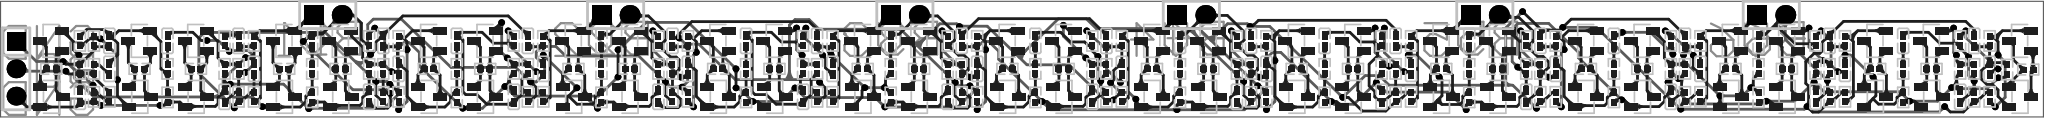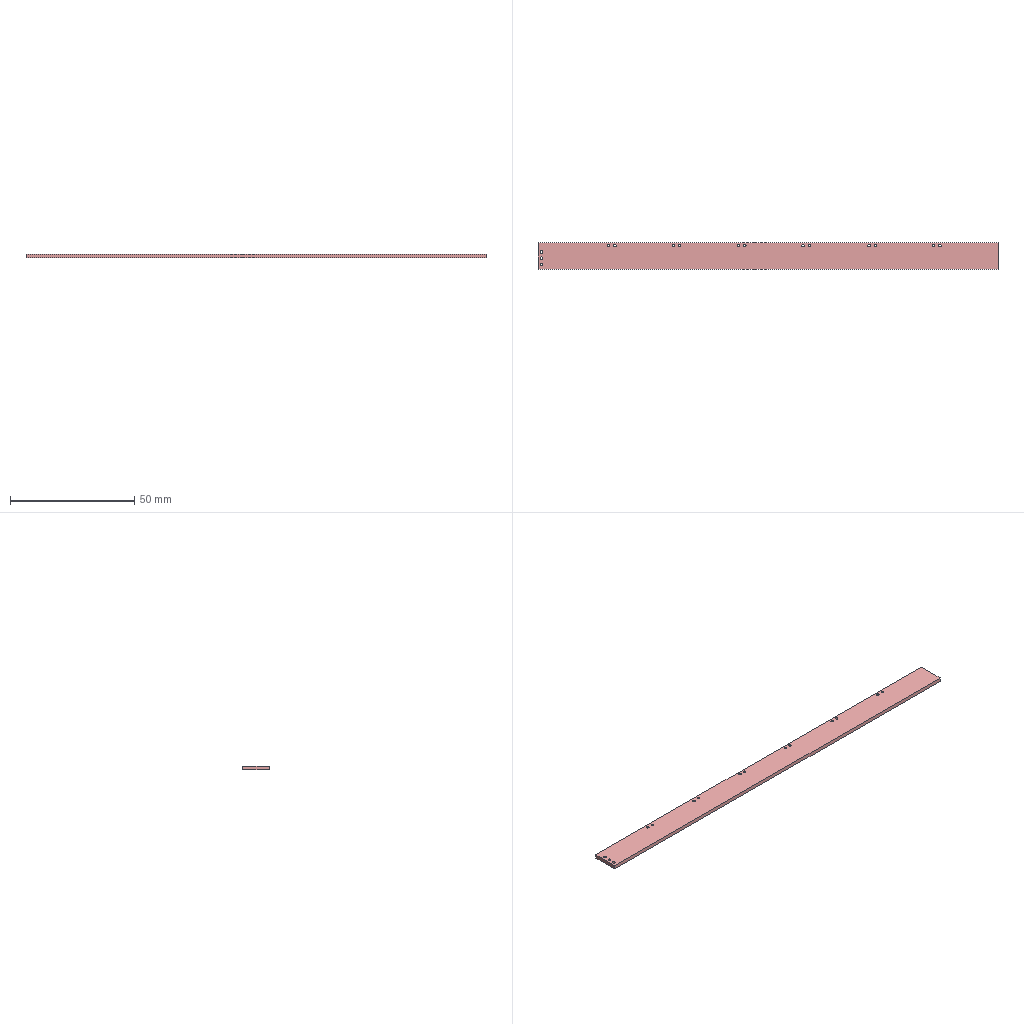Circuit board layout | Altium Designer | box 184.8 x 10.8 x 1.6 mm
Layer stack:
# Altium Designer layer stack of  (unit mm; dielectric type: 0 none, 1 core, 2 prepreg, 3 surface material)
index,name,kind,layer,copper_thickness_mm,dielectric_type,dielectric_thickness_mm,dielectric_material,dielectric_constant
0,Top Paste Mask Layer,other,,,,,,
1,Top Silkscreen Layer,other,,,,,,
2,Top Solder Mask Layer,dielectric,,,3,0.01,,3.3
3,Top Layer,copper,Top Layer,0.035,,,,
4,Dielectric1,dielectric,,,3,1.51,FR4,4.5
5,Bottom Layer,copper,Bottom Layer,0.035,,,,
6,Bottom Solder Mask Layer,dielectric,,,3,0.01,,3.3
7,Bottom Silkscreen Layer,other,,,,,,
8,Bottom Paste Mask Layer,other,,,,,,
# drill layer pairs: low layer,high layer
drill_pair,Top Layer,Bottom Layer
Part placement:
Designator,Comment,Layer,Footprint,Center-X(mm),Center-Y(mm),Rotation
C4,0.1uF,TopLayer,C0402,83.376,80.928,90
C5,0.1uF,TopLayer,C0402,86.043,86.135,270
C2,0.1uF,TopLayer,C0402,86.043,83.531,270
C1,0.1uF,TopLayer,C0402,91.303,86.135,270
C6,0.1uF,TopLayer,C0402,96.457,80.928,270
Q3,MMBT3906,TopLayer,SOT-23-3_L2.9-W1.3-P1.90-LS2.4-BR,80.807,80.928,180
Q2,MMBT3904,TopLayer,SOT-23-3_L2.9-W1.3-P1.90-LS2.4-BR,80.772,86.135,0
Q1,MMBT3906,TopLayer,SOT-23-3_L2.9-W1.3-P1.90-LS2.4-BR,88.755,86.135,0
Q4,MMBT3904,TopLayer,SOT-23-3_L2.9-W1.3-P1.90-LS2.4-BR,88.79,80.928,180
R3,2.2K,TopLayer,R0402,83.376,83.531,90
R4,2.2K,TopLayer,R0402,91.303,80.876,90
Rb1,1K,TopLayer,R0402,80.79,83.531,180
R1,1,TopLayer,R0402,84.645,83.531,270
Rb2,1K,TopLayer,R0402,88.773,83.531,0
R5,1,TopLayer,R0402,91.303,83.531,270
Rp1,200K,TopLayer,R0402,84.645,80.928,90
Rp2,200K,TopLayer,R0402,83.376,86.135,270
Rs1,200,TopLayer,R0402,86.043,80.928,90
Rs2,200,TopLayer,R0402,84.645,86.135,270
C7,0.1uF,TopLayer,C0402,99.124,83.531,270
C8,0.1uF,TopLayer,C0402,97.727,86.135,90
H1,,TopLayer,HDR-TH_3P-P2.54-V-M,77.597,83.531,270
H2,,TopLayer,HDR-TH_2P-P2.54-V-M-1,105.791,88.548,0
H3,,TopLayer,HDR-TH_2P-P2.54-V-M-1,131.826,88.548,0
H4,,TopLayer,HDR-TH_2P-P2.54-V-M-1,157.988,88.548,0
H5,,TopLayer,HDR-TH_2P-P2.54-V-M-1,183.896,88.548,0
H6,,TopLayer,HDR-TH_2P-P2.54-V-M-1,210.439,88.548,0
H7,,TopLayer,HDR-TH_2P-P2.54-V-M-1,236.347,88.548,0
Q5,MMBT3904,TopLayer,SOT-23-3_L2.9-W1.3-P1.90-LS2.4-BR,93.853,86.135,0
Q6,MMBT3906,TopLayer,SOT-23-3_L2.9-W1.3-P1.90-LS2.4-BR,93.888,80.928,180
Q7,MMBT3904,TopLayer,SOT-23-3_L2.9-W1.3-P1.90-LS2.4-BR,101.837,86.135,0
Q8,MMBT3906,TopLayer,SOT-23-3_L2.9-W1.3-P1.90-LS2.4-BR,101.871,80.928,180
R6,1,TopLayer,R0402,96.457,86.135,270
R7,2.2K,TopLayer,R0402,97.727,80.928,270
Rb3,1K,TopLayer,R0402,93.871,83.531,180
Rb4,1K,TopLayer,R0402,101.854,83.531,180
Rp3,200K,TopLayer,R0402,96.457,83.531,90
Rp4,200K,TopLayer,R0402,99.124,86.135,90
Rs3,200,TopLayer,R0402,97.727,83.531,270
Rs4,200,TopLayer,R0402,99.124,80.928,90
C9,0.1uF,TopLayer,C0402,104.384,86.135,270
R8,1,TopLayer,R0402,104.384,83.531,270
R9,2.2K,TopLayer,R0402,104.384,80.876,90
Rb5,1K,TopLayer,R0402,106.951,83.531,180
Q10,MMBT3906,TopLayer,SOT-23-3_L2.9-W1.3-P1.90-LS2.4-BR,106.969,80.928,180
Q9,MMBT3904,TopLayer,SOT-23-3_L2.9-W1.3-P1.90-LS2.4-BR,106.934,86.135,0
Rp5,200K,TopLayer,R0402,109.537,83.531,90
R10,1,TopLayer,R0402,109.537,86.135,270
C10,0.1uF,TopLayer,C0402,109.537,80.928,270
C11,0.1uF,TopLayer,C0402,110.808,86.135,90
R11,2.2K,TopLayer,R0402,110.808,80.928,270
Rs5,200,TopLayer,R0402,110.808,83.531,270
Rs6,200,TopLayer,R0402,112.204,80.928,90
Rp6,200K,TopLayer,R0402,112.204,86.135,90
C12,0.1uF,TopLayer,C0402,112.204,83.531,270
Q12,MMBT3906,TopLayer,SOT-23-3_L2.9-W1.3-P1.90-LS2.4-BR,114.953,80.928,180
Q11,MMBT3904,TopLayer,SOT-23-3_L2.9-W1.3-P1.90-LS2.4-BR,114.918,86.135,0
Rb6,1K,TopLayer,R0402,114.935,83.531,180
C13,0.1uF,TopLayer,C0402,117.465,86.135,270
R12,1,TopLayer,R0402,117.465,83.531,270
R13,2.2K,TopLayer,R0402,117.465,80.876,90
Rb7,1K,TopLayer,R0402,120.032,83.531,180
Q14,MMBT3906,TopLayer,SOT-23-3_L2.9-W1.3-P1.90-LS2.4-BR,120.05,80.928,180
Q13,MMBT3904,TopLayer,SOT-23-3_L2.9-W1.3-P1.90-LS2.4-BR,120.015,86.135,0
Rp7,200K,TopLayer,R0402,122.618,83.531,90
R14,1,TopLayer,R0402,122.618,86.135,270
C14,0.1uF,TopLayer,C0402,122.618,80.928,270
C15,0.1uF,TopLayer,C0402,123.888,86.135,90
R15,2.2K,TopLayer,R0402,123.888,80.928,270
Rs7,200,TopLayer,R0402,123.888,83.531,270
Rs8,200,TopLayer,R0402,125.285,80.928,90
Rp8,200K,TopLayer,R0402,125.285,86.135,90
C16,0.1uF,TopLayer,C0402,125.285,83.531,270
Q16,MMBT3906,TopLayer,SOT-23-3_L2.9-W1.3-P1.90-LS2.4-BR,128.034,80.928,180
Q15,MMBT3904,TopLayer,SOT-23-3_L2.9-W1.3-P1.90-LS2.4-BR,127.999,86.135,0
Rb8,1K,TopLayer,R0402,128.016,83.531,180
C17,0.1uF,TopLayer,C0402,130.546,86.135,270
R16,1,TopLayer,R0402,130.546,83.531,270
R17,2.2K,TopLayer,R0402,130.546,80.876,90
Rb9,1K,TopLayer,R0402,133.113,83.531,180
Q18,MMBT3906,TopLayer,SOT-23-3_L2.9-W1.3-P1.90-LS2.4-BR,133.131,80.928,180
Q17,MMBT3904,TopLayer,SOT-23-3_L2.9-W1.3-P1.90-LS2.4-BR,133.096,86.135,0
Rp9,200K,TopLayer,R0402,135.7,83.531,90
R18,1,TopLayer,R0402,135.7,86.135,270
C18,0.1uF,TopLayer,C0402,135.7,80.928,270
C19,0.1uF,TopLayer,C0402,136.97,86.135,90
R19,2.2K,TopLayer,R0402,136.97,80.928,270
Rs9,200,TopLayer,R0402,136.97,83.531,270
Rs10,200,TopLayer,R0402,138.367,80.928,90
Rp10,200K,TopLayer,R0402,138.367,86.135,90
C20,0.1uF,TopLayer,C0402,138.367,83.531,270
Q20,MMBT3906,TopLayer,SOT-23-3_L2.9-W1.3-P1.90-LS2.4-BR,141.114,80.928,180
Q19,MMBT3904,TopLayer,SOT-23-3_L2.9-W1.3-P1.90-LS2.4-BR,141.079,86.135,0
Rb10,1K,TopLayer,R0402,141.097,83.531,180
C21,0.1uF,TopLayer,C0402,143.627,86.135,270
R20,1,TopLayer,R0402,143.627,83.531,270
R21,2.2K,TopLayer,R0402,143.627,80.876,90
Rb11,1K,TopLayer,R0402,146.195,83.531,180
Q22,MMBT3906,TopLayer,SOT-23-3_L2.9-W1.3-P1.90-LS2.4-BR,146.212,80.928,180
Q21,MMBT3904,TopLayer,SOT-23-3_L2.9-W1.3-P1.90-LS2.4-BR,146.177,86.135,0
Rp11,200K,TopLayer,R0402,148.78,83.531,90
R22,1,TopLayer,R0402,148.78,86.135,270
C22,0.1uF,TopLayer,C0402,148.78,80.928,270
C23,0.1uF,TopLayer,C0402,150.05,86.135,90
R23,2.2K,TopLayer,R0402,150.05,80.928,270
Rs11,200,TopLayer,R0402,150.05,83.531,270
Rs12,200,TopLayer,R0402,151.447,80.928,90
Rp12,200K,TopLayer,R0402,151.447,86.135,90
C24,0.1uF,TopLayer,C0402,151.447,83.531,270
Q24,MMBT3906,TopLayer,SOT-23-3_L2.9-W1.3-P1.90-LS2.4-BR,154.196,80.928,180
Q23,MMBT3904,TopLayer,SOT-23-3_L2.9-W1.3-P1.90-LS2.4-BR,154.161,86.135,0
Rb12,1K,TopLayer,R0402,154.178,83.531,180
C25,0.1uF,TopLayer,C0402,156.708,86.135,270
R24,1,TopLayer,R0402,156.708,83.531,270
R25,2.2K,TopLayer,R0402,156.708,80.876,90
Rb13,1K,TopLayer,R0402,159.275,83.531,180
Q26,MMBT3906,TopLayer,SOT-23-3_L2.9-W1.3-P1.90-LS2.4-BR,159.293,80.928,180
Q25,MMBT3904,TopLayer,SOT-23-3_L2.9-W1.3-P1.90-LS2.4-BR,159.258,86.135,0
Rp13,200K,TopLayer,R0402,161.862,83.531,90
R26,1,TopLayer,R0402,161.862,86.135,270
C26,0.1uF,TopLayer,C0402,161.862,80.928,270
C27,0.1uF,TopLayer,C0402,163.131,86.135,90
R27,2.2K,TopLayer,R0402,163.131,80.928,270
Rs13,200,TopLayer,R0402,163.131,83.531,270
Rs14,200,TopLayer,R0402,164.529,80.928,90
Rp14,200K,TopLayer,R0402,164.529,86.135,90
C28,0.1uF,TopLayer,C0402,164.529,83.531,270
Q28,MMBT3906,TopLayer,SOT-23-3_L2.9-W1.3-P1.90-LS2.4-BR,167.276,80.928,180
Q27,MMBT3904,TopLayer,SOT-23-3_L2.9-W1.3-P1.90-LS2.4-BR,167.242,86.135,0
Rb14,1K,TopLayer,R0402,167.259,83.531,180
C29,0.1uF,TopLayer,C0402,169.789,86.135,270
R28,1,TopLayer,R0402,169.789,83.531,270
R29,2.2K,TopLayer,R0402,169.789,80.876,90
Rb15,1K,TopLayer,R0402,172.357,83.531,180
Q30,MMBT3906,TopLayer,SOT-23-3_L2.9-W1.3-P1.90-LS2.4-BR,172.374,80.928,180
Q29,MMBT3904,TopLayer,SOT-23-3_L2.9-W1.3-P1.90-LS2.4-BR,172.339,86.135,0
Rp15,200K,TopLayer,R0402,174.942,83.531,90
R30,1,TopLayer,R0402,174.942,86.135,270
C30,0.1uF,TopLayer,C0402,174.942,80.928,270
C31,0.1uF,TopLayer,C0402,176.213,86.135,90
R31,2.2K,TopLayer,R0402,176.213,80.928,270
Rs15,200,TopLayer,R0402,176.213,83.531,270
Rs16,200,TopLayer,R0402,177.609,80.928,90
Rp16,200K,TopLayer,R0402,177.609,86.135,90
C32,0.1uF,TopLayer,C0402,177.609,83.531,270
Q32,MMBT3906,TopLayer,SOT-23-3_L2.9-W1.3-P1.90-LS2.4-BR,180.357,80.928,180
Q31,MMBT3904,TopLayer,SOT-23-3_L2.9-W1.3-P1.90-LS2.4-BR,180.322,86.135,0
Rb16,1K,TopLayer,R0402,180.34,83.531,180
C33,0.1uF,TopLayer,C0402,182.87,86.135,270
R32,1,TopLayer,R0402,182.87,83.531,270
R33,2.2K,TopLayer,R0402,182.87,80.876,90
Rb17,1K,TopLayer,R0402,185.438,83.531,180
Q34,MMBT3906,TopLayer,SOT-23-3_L2.9-W1.3-P1.90-LS2.4-BR,185.455,80.928,180
Q33,MMBT3904,TopLayer,SOT-23-3_L2.9-W1.3-P1.90-LS2.4-BR,185.42,86.135,0
Rp17,200K,TopLayer,R0402,188.024,83.531,90
R34,1,TopLayer,R0402,188.024,86.135,270
C34,0.1uF,TopLayer,C0402,188.024,80.928,270
C35,0.1uF,TopLayer,C0402,189.293,86.135,90
R35,2.2K,TopLayer,R0402,189.293,80.928,270
Rs17,200,TopLayer,R0402,189.293,83.531,270
Rs18,200,TopLayer,R0402,190.69,80.928,90
Rp18,200K,TopLayer,R0402,190.69,86.135,90
C36,0.1uF,TopLayer,C0402,190.69,83.531,270
Q36,MMBT3906,TopLayer,SOT-23-3_L2.9-W1.3-P1.90-LS2.4-BR,193.439,80.928,180
Q35,MMBT3904,TopLayer,SOT-23-3_L2.9-W1.3-P1.90-LS2.4-BR,193.404,86.135,0
Rb18,1K,TopLayer,R0402,193.421,83.531,180
C37,0.1uF,TopLayer,C0402,195.951,86.135,270
R36,1,TopLayer,R0402,195.951,83.531,270
R37,2.2K,TopLayer,R0402,195.951,80.876,90
Rb19,1K,TopLayer,R0402,198.518,83.531,180
Q38,MMBT3906,TopLayer,SOT-23-3_L2.9-W1.3-P1.90-LS2.4-BR,198.536,80.928,180
Q37,MMBT3904,TopLayer,SOT-23-3_L2.9-W1.3-P1.90-LS2.4-BR,198.501,86.135,0
Rp19,200K,TopLayer,R0402,201.105,83.531,90
R38,1,TopLayer,R0402,201.105,86.135,270
C38,0.1uF,TopLayer,C0402,201.105,80.928,270
C39,0.1uF,TopLayer,C0402,202.375,86.135,90
R39,2.2K,TopLayer,R0402,202.375,80.928,270
Rs19,200,TopLayer,R0402,202.375,83.531,270
Rs20,200,TopLayer,R0402,203.772,80.928,90
Rp20,200K,TopLayer,R0402,203.772,86.135,90
C40,0.1uF,TopLayer,C0402,203.772,83.531,270
Q40,MMBT3906,TopLayer,SOT-23-3_L2.9-W1.3-P1.90-LS2.4-BR,206.519,80.928,180
Q39,MMBT3904,TopLayer,SOT-23-3_L2.9-W1.3-P1.90-LS2.4-BR,206.484,86.135,0
Rb20,1K,TopLayer,R0402,206.502,83.531,180
C41,0.1uF,TopLayer,C0402,209.032,86.135,270
R40,1,TopLayer,R0402,209.032,83.531,270
R41,2.2K,TopLayer,R0402,209.032,80.876,90
Rb21,1K,TopLayer,R0402,211.6,83.531,180
Q42,MMBT3906,TopLayer,SOT-23-3_L2.9-W1.3-P1.90-LS2.4-BR,211.617,80.928,180
Q41,MMBT3904,TopLayer,SOT-23-3_L2.9-W1.3-P1.90-LS2.4-BR,211.582,86.135,0
Rp21,200K,TopLayer,R0402,214.185,83.531,90
R42,1,TopLayer,R0402,214.185,86.135,270
C42,0.1uF,TopLayer,C0402,214.185,80.928,270
C43,0.1uF,TopLayer,C0402,215.456,86.135,90
R43,2.2K,TopLayer,R0402,215.456,80.928,270
Rs21,200,TopLayer,R0402,215.456,83.531,270
Rs22,200,TopLayer,R0402,216.852,80.928,90
Rp22,200K,TopLayer,R0402,216.852,86.135,90
C44,0.1uF,TopLayer,C0402,216.852,83.531,270
Q44,MMBT3906,TopLayer,SOT-23-3_L2.9-W1.3-P1.90-LS2.4-BR,219.601,80.928,180
Q43,MMBT3904,TopLayer,SOT-23-3_L2.9-W1.3-P1.90-LS2.4-BR,219.565,86.135,0
Rb22,1K,TopLayer,R0402,219.583,83.531,180
C45,0.1uF,TopLayer,C0402,222.113,86.135,270
R44,1,TopLayer,R0402,222.113,83.531,270
R45,2.2K,TopLayer,R0402,222.113,80.876,90
Rb23,1K,TopLayer,R0402,224.68,83.531,180
Q46,MMBT3906,TopLayer,SOT-23-3_L2.9-W1.3-P1.90-LS2.4-BR,224.698,80.928,180
Q45,MMBT3904,TopLayer,SOT-23-3_L2.9-W1.3-P1.90-LS2.4-BR,224.663,86.135,0
Rp23,200K,TopLayer,R0402,227.267,83.531,90
R46,1,TopLayer,R0402,227.267,86.135,270
C46,0.1uF,TopLayer,C0402,227.267,80.928,270
C47,0.1uF,TopLayer,C0402,228.536,86.135,90
R47,2.2K,TopLayer,R0402,228.536,80.928,270
Rs23,200,TopLayer,R0402,228.536,83.531,270
Rs24,200,TopLayer,R0402,229.934,80.928,90
Rp24,200K,TopLayer,R0402,229.934,86.135,90
C48,0.1uF,TopLayer,C0402,229.934,83.531,270
Q48,MMBT3906,TopLayer,SOT-23-3_L2.9-W1.3-P1.90-LS2.4-BR,232.681,80.928,180
Q47,MMBT3904,TopLayer,SOT-23-3_L2.9-W1.3-P1.90-LS2.4-BR,232.646,86.135,0
Rb24,1K,TopLayer,R0402,232.664,83.531,180
C49,0.1uF,TopLayer,C0402,235.194,86.135,270
R48,1,TopLayer,R0402,235.194,83.531,270
R49,2.2K,TopLayer,R0402,235.194,80.876,90
Rb25,1K,TopLayer,R0402,237.762,83.531,180
Q50,MMBT3906,TopLayer,SOT-23-3_L2.9-W1.3-P1.90-LS2.4-BR,237.779,80.928,180
Q49,MMBT3904,TopLayer,SOT-23-3_L2.9-W1.3-P1.90-LS2.4-BR,237.744,86.135,0
Rp25,200K,TopLayer,R0402,240.347,83.531,90
R50,1,TopLayer,R0402,240.347,86.135,270
C50,0.1uF,TopLayer,C0402,240.347,80.928,270
C51,0.1uF,TopLayer,C0402,241.618,86.135,90
R51,2.2K,TopLayer,R0402,241.618,80.928,270
Rs25,200,TopLayer,R0402,241.618,83.531,270
Rs26,200,TopLayer,R0402,243.014,80.928,90
Rp26,200K,TopLayer,R0402,243.014,86.135,90
C52,0.1uF,TopLayer,C0402,243.014,83.531,270
Q52,MMBT3906,TopLayer,SOT-23-3_L2.9-W1.3-P1.90-LS2.4-BR,245.762,80.928,180
Q51,MMBT3904,TopLayer,SOT-23-3_L2.9-W1.3-P1.90-LS2.4-BR,245.727,86.135,0
Rb26,1K,TopLayer,R0402,245.745,83.531,180
C53,0.1uF,TopLayer,C0402,248.275,86.135,270
R52,1,TopLayer,R0402,248.275,83.531,270
R53,2.2K,TopLayer,R0402,248.275,80.876,90
Rb27,1K,TopLayer,R0402,250.843,83.531,180
Q54,MMBT3906,TopLayer,SOT-23-3_L2.9-W1.3-P1.90-LS2.4-BR,250.86,80.928,180
Q53,MMBT3904,TopLayer,SOT-23-3_L2.9-W1.3-P1.90-LS2.4-BR,250.825,86.135,0
Rp27,200K,TopLayer,R0402,253.429,83.531,90
R54,1,TopLayer,R0402,253.429,86.135,270
C54,0.1uF,TopLayer,C0402,253.429,80.928,270
C55,0.1uF,TopLayer,C0402,254.698,86.135,90
R55,2.2K,TopLayer,R0402,254.698,80.928,270
Rs27,200,TopLayer,R0402,254.698,83.531,270
Rs28,200,TopLayer,R0402,256.096,80.928,90
Rp28,200K,TopLayer,R0402,256.096,86.135,90
C56,0.1uF,TopLayer,C0402,256.096,83.531,270
Q56,MMBT3906,TopLayer,SOT-23-3_L2.9-W1.3-P1.90-LS2.4-BR,258.844,80.928,180
Q55,MMBT3904,TopLayer,SOT-23-3_L2.9-W1.3-P1.90-LS2.4-BR,258.808,86.135,0
Rb28,1K,TopLayer,R0402,259.588,83.468,180
R56,2.2K,TopLayer,R0402,257.683,83.468,90
Pad and via stacks:
# Altium Designer via and pad stacks of  (unit mm). Each distinct definition once, with the count of objects using it.
# via: kind,start_layer,end_layer,hole_mm,diameter_mm,mode(0 simple;1 top-mid-bottom;2 full stack),diameter_per_layer,count,example_net
# pad: kind,layer,hole_mm,hole_type(0 round;1 square;2 slot),plating,top_size,top_shape(1 round;2 rect;3 octagon;9 rounded rect),mid_size,bottom_size,mode,footprint,size_per_layer,count,example
pad,Top Layer,0,0,plated,0.7901x0.54,2,0.7901x0.54,0.7901x0.54,0,C0402,,110,C4.2
pad,Top Layer,0,0,plated,1.25x0.7,2,1.25x0.7,1.25x0.7,0,SOT-23-3_L2.9-W1.3-P1.90-LS2.4-BR,,168,Q3.1
pad,Top Layer,0,0,plated,0.5657x0.54,2,0.5657x0.54,0.5657x0.54,0,R0402,,278,R3.2
pad,Multi-Layer,1.1,0,plated,1.7x1.7,2,1.7x1.7,1.7x1.7,0,HDR-TH_3P-P2.54-V-M,,1,H1.1
pad,Multi-Layer,1.1,0,plated,1.7x1.7,1,1.7x1.7,1.7x1.7,0,HDR-TH_3P-P2.54-V-M,,2,H1.2
pad,Multi-Layer,1,0,plated,1.8x1.8,1,1.8x1.8,1.8x1.8,0,HDR-TH_2P-P2.54-V-M-1,,6,H2.2
pad,Multi-Layer,1,0,plated,1.8x1.8,2,1.8x1.8,1.8x1.8,0,HDR-TH_2P-P2.54-V-M-1,,6,H2.1
via,Top Layer,Bottom Layer,0.3048,0.61,0,,133,$1N10366